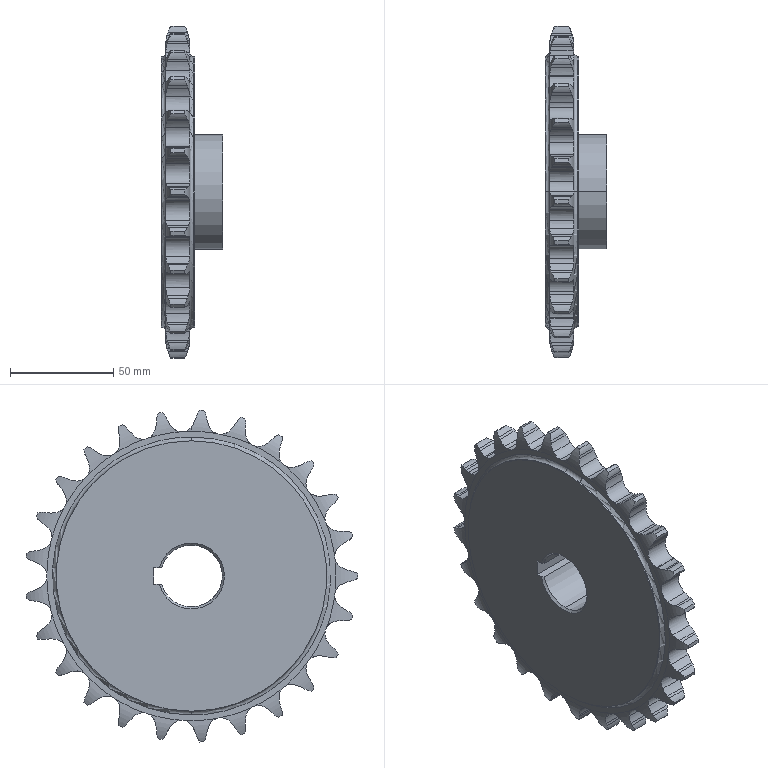Part | NX | features BREP 1 | 1 solid | 290 faces | box 30 x 160.481 x 160.793 mm | volume 272453 mm3 | cylinder 171 | plane 58 | torus 56 | cone 5 | commonest cylinder face diameters 17.202 x53 31.126 x52 12.07 x32 161 x25 131 x4 30 x3